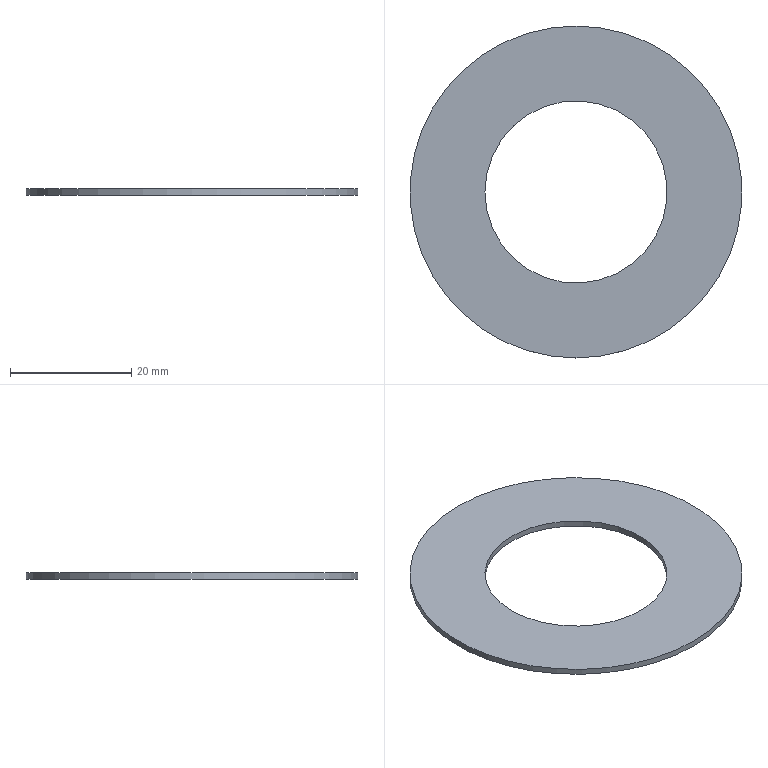Part | NX | features solid 2 | 1 solid | 4 faces | box 54.687 x 54.687 x 1 mm | volume 1642 mm3 | cylinder 2 | plane 2 | commonest cylinder face diameters 30 x1 54.687 x1
STEP:
#1=CARTESIAN_POINT('',(-15.,-440.,-124.));
#2=VERTEX_POINT('',#1);
#3=CARTESIAN_POINT('',(0.,-440.,-124.));
#4=DIRECTION('',(0.,0.,1.));
#5=DIRECTION('',(-1.,0.,0.));
#6=AXIS2_PLACEMENT_3D('',#3,#4,#5);
#7=CIRCLE('',#6,15.);
#8=EDGE_CURVE('',#2,#2,#7,.T.);
#9=ORIENTED_EDGE('',*,*,#8,.T.);
#10=EDGE_LOOP('',(#9));
#11=FACE_BOUND('',#10,.T.);
#12=CARTESIAN_POINT('',(-15.,-440.,-125.));
#13=VERTEX_POINT('',#12);
#14=CARTESIAN_POINT('',(0.,-440.,-125.));
#15=DIRECTION('',(0.,0.,1.));
#16=DIRECTION('',(-1.,0.,0.));
#17=AXIS2_PLACEMENT_3D('',#14,#15,#16);
#18=CIRCLE('',#17,15.);
#19=EDGE_CURVE('',#13,#13,#18,.T.);
#20=ORIENTED_EDGE('',*,*,#19,.F.);
#21=EDGE_LOOP('',(#20));
#22=FACE_BOUND('',#21,.T.);
#23=CARTESIAN_POINT('',(0.,-440.,-124.));
#24=DIRECTION('',(0.,0.,-1.));
#25=DIRECTION('',(1.,0.,0.));
#26=AXIS2_PLACEMENT_3D('',#23,#24,#25);
#27=CYLINDRICAL_SURFACE('',#26,15.);
#28=ADVANCED_FACE('',(#11,#22),#27,.F.);
#29=CARTESIAN_POINT('',(0.,-467.343,-124.));
#30=VERTEX_POINT('',#29);
#31=CARTESIAN_POINT('',(0.,-440.,-124.));
#32=DIRECTION('',(0.,0.,1.));
#33=DIRECTION('',(0.,-1.,0.));
#34=AXIS2_PLACEMENT_3D('',#31,#32,#33);
#35=CIRCLE('',#34,27.343);
#36=EDGE_CURVE('',#30,#30,#35,.T.);
#37=ORIENTED_EDGE('',*,*,#36,.F.);
#38=EDGE_LOOP('',(#37));
#39=FACE_BOUND('',#38,.T.);
#40=CARTESIAN_POINT('',(0.,-467.343,-125.));
#41=VERTEX_POINT('',#40);
#42=CARTESIAN_POINT('',(0.,-440.,-125.));
#43=DIRECTION('',(0.,0.,1.));
#44=DIRECTION('',(0.,-1.,0.));
#45=AXIS2_PLACEMENT_3D('',#42,#43,#44);
#46=CIRCLE('',#45,27.343);
#47=EDGE_CURVE('',#41,#41,#46,.T.);
#48=ORIENTED_EDGE('',*,*,#47,.T.);
#49=EDGE_LOOP('',(#48));
#50=FACE_BOUND('',#49,.T.);
#51=CARTESIAN_POINT('',(0.,-440.,-124.));
#52=DIRECTION('',(0.,0.,-1.));
#53=DIRECTION('',(1.,0.,0.));
#54=AXIS2_PLACEMENT_3D('',#51,#52,#53);
#55=CYLINDRICAL_SURFACE('',#54,27.343);
#56=ADVANCED_FACE('',(#39,#50),#55,.T.);
#57=ORIENTED_EDGE('',*,*,#8,.F.);
#58=EDGE_LOOP('',(#57));
#59=FACE_BOUND('',#58,.T.);
#60=ORIENTED_EDGE('',*,*,#36,.T.);
#61=EDGE_LOOP('',(#60));
#62=FACE_BOUND('',#61,.T.);
#63=CARTESIAN_POINT('',(0.,-440.,-124.));
#64=DIRECTION('',(0.,0.,-1.));
#65=DIRECTION('',(1.,0.,0.));
#66=AXIS2_PLACEMENT_3D('',#63,#64,#65);
#67=PLANE('',#66);
#68=ADVANCED_FACE('',(#59,#62),#67,.F.);
#69=ORIENTED_EDGE('',*,*,#19,.T.);
#70=EDGE_LOOP('',(#69));
#71=FACE_BOUND('',#70,.T.);
#72=ORIENTED_EDGE('',*,*,#47,.F.);
#73=EDGE_LOOP('',(#72));
#74=FACE_BOUND('',#73,.T.);
#75=CARTESIAN_POINT('',(0.,-440.,-125.));
#76=DIRECTION('',(0.,0.,-1.));
#77=DIRECTION('',(1.,0.,0.));
#78=AXIS2_PLACEMENT_3D('',#75,#76,#77);
#79=PLANE('',#78);
#80=ADVANCED_FACE('',(#71,#74),#79,.T.);
#81=CLOSED_SHELL('',(#28,#56,#68,#80));
#82=MANIFOLD_SOLID_BREP('',#81);
#83=(LENGTH_UNIT()NAMED_UNIT(*)SI_UNIT(.MILLI.,.METRE.));
#84=UNCERTAINTY_MEASURE_WITH_UNIT(LENGTH_MEASURE(0.00001),#83,'','');
#85=(NAMED_UNIT(*)PLANE_ANGLE_UNIT()SI_UNIT($,.RADIAN.));
#86=(NAMED_UNIT(*)SI_UNIT($,.STERADIAN.)SOLID_ANGLE_UNIT());
#87=(GEOMETRIC_REPRESENTATION_CONTEXT(3)GLOBAL_UNCERTAINTY_ASSIGNED_CONTEXT((#84))GLOBAL_UNIT_ASSIGNED_CONTEXT((#83,#85,#86))REPRESENTATION_CONTEXT('',''));
#88=ADVANCED_BREP_SHAPE_REPRESENTATION('',(#82),#87);